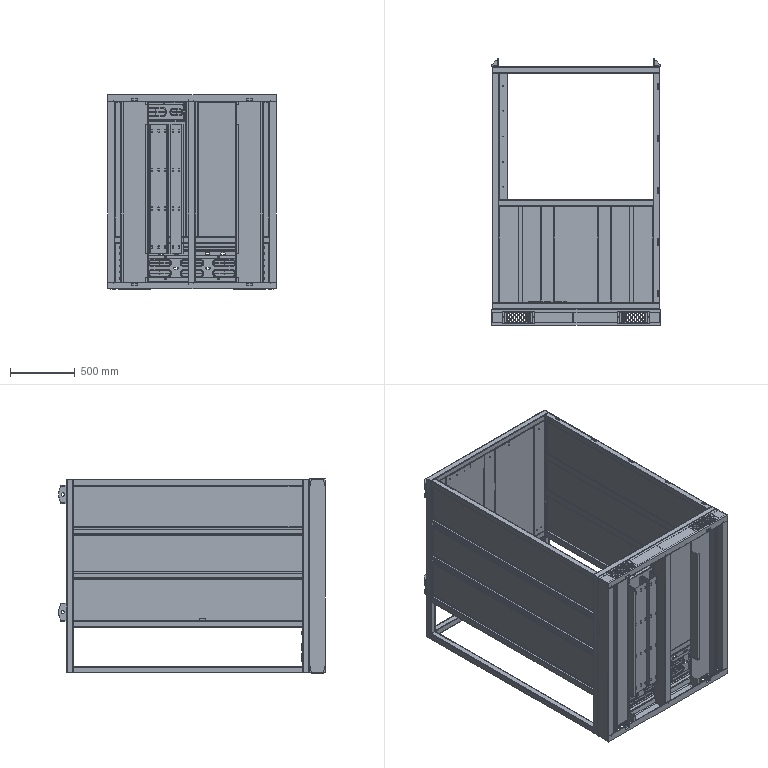Part | SolidWorks | 85 solids | 4216 faces | volume 55834819 mm3 | plane 2833 | cylinder 1375 | torus 8 | commonest cylinder face diameters 12 x224 15 x115 10 x104 6 x95 1.473 x85 6.473 x85